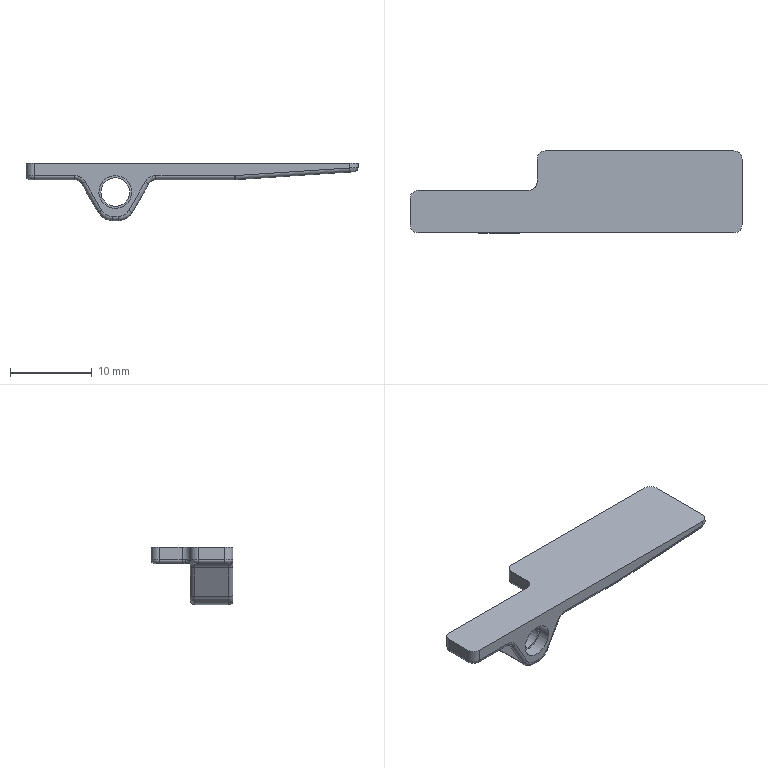NC program | Mastercam | posted with a generic post | part box 40.5 x 10 x 7 mm
Lines 1 to 1263 of 12178:
%
:0001()
(MATERIAL - ALUMINUM MM - 2024)
(T10|10 FEM |H10)
(T2|2 FEM |H2)
(T20|63 FEM |H20)
(T7|4 CHM |H7)
(T3|3 FEM |H3)
(T6|6 FEM |H6)
(T1|2 BM/BNOS |H1)
N100 G21
N102 G0 G17 G40 G80 G90 G94 G98
N104 G0 G28 G91 Z0.
N106 G0 G28 X0. Y0.
(10 FEM |TOOL - 10|DIA. OFF. - 10|LEN. - 10|TOOL DIA. - 10.)
N108 T10 M6
N110 G0 G54 G90 X20.25 Y-12. C0. B0. S6500 M3
N112 G43 H10 Z50.
N114 Z1.
N116 G1 Z-7. F600.
N118 Y-11. F1000.
N120 G3 X19.25 Y-10. I-1.
N122 G1 X-19.25
N124 G2 X-25.25 Y-4. J6.
N126 G1 Y-.8
N128 G2 X-19.25 Y5.2 I6.
N130 G1 X-9.629
N132 G2 X-3.75 Y10. I5.879 J-1.2
N134 G1 X19.25
N136 G2 X25.25 Y4. J-6.
N138 G1 Y-4.
N140 G2 X19.25 Y-10. I-6.
N142 G1 X18.75
N144 G3 X17.75 Y-11. J-1.
N146 G1 Y-12.
N148 G0 Z50.
N150 M5
N152 G0 G28 G91 Z0.
N154 G28
N156 M01
N158 G0 G17 G40 G80 G90 G94 G98
N160 G0 G28 G91 Z0.
(2 FEM |TOOL - 2|DIA. OFF. - 2|LEN. - 2|TOOL DIA. - 2.)
N162 T2 M6
N164 G0 G54 G90 X-10.121 Y1.6 C0. B0. S5000 M3
N166 G43 H2 Z50.
N168 Z1.
N170 G1 Z-7. F600.
N172 Y1.4
N174 G3 X-9.921 Y1.2 I.2
N176 G1 X-5.75
N178 Y4.
N180 G2 X-5.507 Y4.955 I2.
N182 G3 X-5.483 Y5.05 I-.176 J.095
N184 X-5.588 Y5.226 I-.2
N186 G1 X-5.764 Y5.321
N188 G0 Z50.
N190 M5
N192 G0 G28 G91 Z0.
N194 G28
N196 M01
N198 G0 G17 G40 G80 G90 G94 G98
N200 G0 G28 G91 Z0.
(63 FEM |TOOL - 20|DIA. OFF. - 20|LEN. - 20|TOOL DIA. - 63.)
N202 T20 M6
N204 G0 G54 G90 X0. Y-65.2 C0. B0. S4000 M3
N206 G43 H20 Z55.
N208 Z7.
N210 G1 Z4.623 F600.
N212 Y65.2 F2000.
N214 G0 Z54.623
N216 Y-65.2
N218 Z6.623
N220 G1 Z4.246 F600.
N222 Y65.2 F2000.
N224 G0 Z54.246
N226 Y-65.2
N228 Z6.246
N230 G1 Z3.869 F600.
N232 Y65.2 F2000.
N234 G0 Z53.869
N236 Y-65.2
N238 Z5.869
N240 G1 Z3.492 F600.
N242 Y65.2 F2000.
N244 G0 Z53.492
N246 Y-65.2
N248 Z5.492
N250 G1 Z3.115 F600.
N252 Y65.2 F2000.
N254 G0 Z53.115
N256 Y-65.2
N258 Z5.115
N260 G1 Z2.738 F600.
N262 Y65.2 F2000.
N264 G0 Z52.738
N266 Y-65.2
N268 Z4.738
N270 G1 Z2.362 F600.
N272 Y65.2 F2000.
N274 G0 Z52.362
N276 Y-65.2
N278 Z4.362
N280 G1 Z1.985 F600.
N282 Y65.2 F2000.
N284 G0 Z51.985
N286 Y-65.2
N288 Z3.985
N290 G1 Z1.608 F600.
N292 Y65.2 F2000.
N294 G0 Z51.608
N296 Y-65.2
N298 Z3.608
N300 G1 Z1.231 F600.
N302 Y65.2 F2000.
N304 G0 Z51.231
N306 Y-65.2
N308 Z3.231
N310 G1 Z.854 F600.
N312 Y65.2 F2000.
N314 G0 Z50.854
N316 Y-65.2
N318 Z2.854
N320 G1 Z.477 F600.
N322 Y65.2 F2000.
N324 G0 Z50.477
N326 Y-65.2
N328 Z2.477
N330 G1 Z.1 F600.
N332 Y65.2 F2000.
N334 G0 Z50.1
N336 Y-65.2
N338 Z2.1
N340 G1 Z0. F600.
N342 Y65.2 F1000.
N344 G0 Z50.
N346 M5
N348 G0 G28 G91 Z0.
N350 G28
N352 M01
N354 G0 G17 G40 G80 G90 G94 G98
N356 G0 G28 G91 Z0.
(4 CHM |TOOL - 7|DIA. OFF. - 7|LEN. - 7|TOOL DIA. - 4.)
N358 T7 M6
N360 G0 G54 G90 X19.65 Y-6.45 C0. B0. S6500 M3
N362 G43 H7 Z50.
N364 Z1.
N366 G1 Z-.7 F600.
N368 Y-6.05 F1000.
N370 G3 X19.25 Y-5.65 I-.4
N372 G1 X-3.75
N374 G2 X-5.4 Y-4. J1.65
N376 G1 Y-1.2
N378 G3 X-5.75 Y-.85 I-.35
N380 G1 X-19.25
N382 G2 X-20.9 Y.8 J1.65
N384 G1 Y4.
N386 G2 X-19.25 Y5.65 I1.65
N388 G1 X19.25
N390 G2 X20.9 Y4. J-1.65
N392 G1 Y-4.
N394 G2 X19.25 Y-5.65 I-1.65
N396 G3 X18.85 Y-6.05 J-.4
N398 G1 Y-6.45
N400 G0 Z50.
N402 M5
N404 G0 G28 G91 Z0.
N406 G28
N408 M01
N410 G0 G17 G40 G80 G90 G94 G98
N412 G0 G28 G91 Z0.
(3 FEM |TOOL - 3|DIA. OFF. - 3|LEN. - 3|TOOL DIA. - 3.)
N414 T3 M6
N416 G0 G54 G90 X-9.097 Y-.334 C0. B0. S6000 M3
N418 G43 H3 Z50.
N420 Z2.5
N422 G1 Z2. F600.
N424 X-9.091 Y-.33 Z1.839 F1000.
N426 X-9.075 Y-.321 Z1.68
N428 X-9.05 Y-.287 Z1.487
N430 X-9.015 Y-.239 Z1.299
N432 X-8.969 Y-.176 Z1.118
N434 X-8.952 Y-.094 Z.966
N436 X-8.932 Y0. Z.821
N438 X-8.95 Y.084 Z.711
N440 X-8.969 Y.176 Z.607
N442 X-9.021 Y.246 Z.523
N444 X-9.075 Y.321 Z.444
N446 X-9.148 Y.374 Z.375
N448 X-9.231 Y.401 Z.316
N450 X-9.318 Y.429 Z.261
N452 X-9.408 Z.212
N454 X-9.579 Y.374 Z.133
N456 X-9.712 Y.254 Z.074
N458 X-9.785 Y.089 Z.032
N460 Y-.089 Z.008
N462 X-9.712 Y-.254 Z0.
N464 X-9.579 Y-.374
N466 X-9.368 Y-.438
N468 X-9.23 Y-.41
N470 X-9.075 Y-.321
N472 X-8.969 Y-.176
N474 X-8.932 Y0.
N476 X-8.969 Y.176
N478 X-9.075 Y.321
N480 X-9.148 Y.374
N482 X-9.318 Y.429
N484 X-9.408
N486 X-9.579 Y.374
N488 X-9.712 Y.254
N490 X-9.785 Y.089
N492 Y-.089
N494 X-9.712 Y-.254
N496 X-9.587 Y-.366 Z-.016
N498 X-9.549 Y-.383 Z-.019
N500 X-9.388 Y-.432 Z-.035
N502 X-9.347 Y-.433 Z-.039
N504 X-9.265 Y-.417 Z-.047
N506 X-9.224 Y-.407 Z-.051
N508 X-9.078 Y-.323 Z-.066
N510 X-9.052 Y-.29 Z-.07
N512 X-8.978 Y-.188 Z-.082
N514 X-8.964 Y-.149 Z-.086
N516 X-8.937 Y-.026 Z-.098
N518 X-8.935 Y.015 Z-.101
N520 X-8.962 Y.139 Z-.113
N522 X-8.972 Y.179 Z-.117
N524 X-9.071 Y.316 Z-.133
N526 X-9.104 Y.342 Z-.137
N528 X-9.138 Y.366 Z-.141
N530 X-9.176 Y.383 Z-.144
N532 X-9.296 Y.422 Z-.156
N534 X-9.337 Y.429 Z-.16
N536 X-9.379 Z-.164
N538 X-9.421 Y.425 Z-.168
N540 X-9.541 Y.386 Z-.18
N542 X-9.58 Y.372 Z-.184
N544 X-9.705 Y.26 Z-.199
N546 X-9.726 Y.223 Z-.203
N548 X-9.777 Y.108 Z-.215
N550 X-9.785 Y.068 Z-.219
N552 Y-.059 Z-.23
N554 X-9.781 Y-.1 Z-.234
N556 X-9.712 Y-.254 Z-.25
N558 X-9.587 Y-.366 Z-.266
N560 X-9.549 Y-.383 Z-.269
N562 X-9.388 Y-.432 Z-.285
N564 X-9.347 Y-.433 Z-.289
N566 X-9.265 Y-.417 Z-.297
N568 X-9.224 Y-.407 Z-.301
N570 X-9.078 Y-.323 Z-.316
N572 X-9.052 Y-.29 Z-.32
N574 X-8.978 Y-.188 Z-.332
N576 X-8.964 Y-.149 Z-.336
N578 X-8.937 Y-.026 Z-.348
N580 X-8.935 Y.015 Z-.351
N582 X-8.962 Y.139 Z-.363
N584 X-8.972 Y.179 Z-.367
N586 X-9.071 Y.316 Z-.383
N588 X-9.104 Y.342 Z-.387
N590 X-9.138 Y.366 Z-.391
N592 X-9.176 Y.383 Z-.394
N594 X-9.296 Y.422 Z-.406
N596 X-9.337 Y.429 Z-.41
N598 X-9.379 Z-.414
N600 X-9.421 Y.425 Z-.418
N602 X-9.541 Y.386 Z-.43
N604 X-9.58 Y.372 Z-.434
N606 X-9.705 Y.26 Z-.449
N608 X-9.726 Y.223 Z-.453
N610 X-9.777 Y.108 Z-.465
N612 X-9.785 Y.068 Z-.469
N614 Y-.059 Z-.48
N616 X-9.781 Y-.1 Z-.484
N618 X-9.712 Y-.254 Z-.5
N620 X-9.587 Y-.366 Z-.516
N622 X-9.549 Y-.383 Z-.519
N624 X-9.388 Y-.432 Z-.535
N626 X-9.347 Y-.433 Z-.539
N628 X-9.265 Y-.417 Z-.547
N630 X-9.224 Y-.407 Z-.551
N632 X-9.078 Y-.323 Z-.566
N634 X-9.052 Y-.29 Z-.57
N636 X-8.978 Y-.188 Z-.582
N638 X-8.964 Y-.149 Z-.586
N640 X-8.937 Y-.026 Z-.598
N642 X-8.935 Y.015 Z-.601
N644 X-8.962 Y.139 Z-.613
N646 X-8.972 Y.179 Z-.617
N648 X-9.071 Y.316 Z-.633
N650 X-9.104 Y.342 Z-.637
N652 X-9.138 Y.366 Z-.641
N654 X-9.176 Y.383 Z-.644
N656 X-9.296 Y.422 Z-.656
N658 X-9.337 Y.429 Z-.66
N660 X-9.379 Z-.664
N662 X-9.421 Y.425 Z-.668
N664 X-9.541 Y.386 Z-.68
N666 X-9.58 Y.372 Z-.684
N668 X-9.705 Y.26 Z-.699
N670 X-9.726 Y.223 Z-.703
N672 X-9.777 Y.108 Z-.715
N674 X-9.785 Y.068 Z-.719
N676 Y-.059 Z-.73
N678 X-9.781 Y-.1 Z-.734
N680 X-9.712 Y-.254 Z-.75
N682 X-9.587 Y-.366 Z-.766
N684 X-9.549 Y-.383 Z-.769
N686 X-9.388 Y-.432 Z-.785
N688 X-9.347 Y-.433 Z-.789
N690 X-9.265 Y-.417 Z-.797
N692 X-9.224 Y-.407 Z-.801
N694 X-9.078 Y-.323 Z-.816
N696 X-9.052 Y-.29 Z-.82
N698 X-8.978 Y-.188 Z-.832
N700 X-8.964 Y-.149 Z-.836
N702 X-8.937 Y-.026 Z-.848
N704 X-8.935 Y.015 Z-.851
N706 X-8.962 Y.139 Z-.863
N708 X-8.972 Y.179 Z-.867
N710 X-9.071 Y.316 Z-.883
N712 X-9.104 Y.342 Z-.887
N714 X-9.138 Y.366 Z-.891
N716 X-9.176 Y.383 Z-.894
N718 X-9.296 Y.422 Z-.906
N720 X-9.337 Y.429 Z-.91
N722 X-9.379 Z-.914
N724 X-9.421 Y.425 Z-.918
N726 X-9.541 Y.386 Z-.93
N728 X-9.58 Y.372 Z-.934
N730 X-9.705 Y.26 Z-.949
N732 X-9.726 Y.223 Z-.953
N734 X-9.777 Y.108 Z-.965
N736 X-9.785 Y.068 Z-.969
N738 Y-.059 Z-.98
N740 X-9.781 Y-.1 Z-.984
N742 X-9.712 Y-.254 Z-1.
N744 X-9.587 Y-.366 Z-1.016
N746 X-9.549 Y-.383 Z-1.019
N748 X-9.388 Y-.432 Z-1.035
N750 X-9.347 Y-.433 Z-1.039
N752 X-9.265 Y-.417 Z-1.047
N754 X-9.224 Y-.407 Z-1.051
N756 X-9.078 Y-.323 Z-1.066
N758 X-9.052 Y-.29 Z-1.07
N760 X-8.978 Y-.188 Z-1.082
N762 X-8.964 Y-.149 Z-1.086
N764 X-8.937 Y-.026 Z-1.098
N766 X-8.935 Y.015 Z-1.101
N768 X-8.962 Y.139 Z-1.113
N770 X-8.972 Y.179 Z-1.117
N772 X-9.071 Y.316 Z-1.133
N774 X-9.104 Y.342 Z-1.137
N776 X-9.138 Y.366 Z-1.141
N778 X-9.176 Y.383 Z-1.144
N780 X-9.296 Y.422 Z-1.156
N782 X-9.337 Y.429 Z-1.16
N784 X-9.379 Z-1.164
N786 X-9.421 Y.425 Z-1.168
N788 X-9.541 Y.386 Z-1.18
N790 X-9.58 Y.372 Z-1.184
N792 X-9.705 Y.26 Z-1.199
N794 X-9.726 Y.223 Z-1.203
N796 X-9.777 Y.108 Z-1.215
N798 X-9.785 Y.068 Z-1.219
N800 Y-.059 Z-1.23
N802 X-9.781 Y-.1 Z-1.234
N804 X-9.712 Y-.254 Z-1.25
N806 X-9.578 Y-.353 Z-1.266
N808 X-9.54 Y-.366 Z-1.27
N810 X-9.502 Y-.374 Z-1.273
N812 X-9.421 Y-.39 Z-1.281
N814 X-9.386 Y-.397 Z-1.285
N816 X-9.351 Y-.394 Z-1.288
N818 X-9.237 Y-.357 Z-1.301
N820 X-9.122 Y-.271 Z-1.316
N822 X-9.099 Y-.239 Z-1.32
N824 X-9.053 Y-.153 Z-1.331
N826 X-9.041 Y-.113 Z-1.336
N828 X-9.035 Y-.026 Z-1.347
N830 X-9.037 Y.015 Z-1.352
N832 X-9.055 Y.072 Z-1.359
N834 X-9.08 Y.129 Z-1.367
N836 X-9.121 Y.179 Z-1.375
N838 X-9.158 Y.213 Z-1.381
N840 X-9.193 Y.237 Z-1.387
N842 X-9.217 Y.25 Z-1.391
N844 X-9.322 Y.264 Z-1.405
N846 X-9.387 Y.265 Z-1.414
N848 X-9.476 Y.22 Z-1.43
N850 X-9.501 Y.198 Z-1.435
N852 X-9.534 Y.155 Z-1.445
N854 X-9.555 Y.116 Z-1.452
N856 X-9.551 Y.077 Z-1.459
N858 X-9.557 Y.022 Z-1.469
N860 X-9.552 Y.01 Z-1.471
N862 X-9.547 Y-.032 Z-1.479
N864 X-9.539 Y-.06 Z-1.484
N866 X-9.537 Z-1.485
N868 X-9.532 Y-.071 Z-1.487
N870 X-9.528 Y-.078 Z-1.489
N872 X-9.52 Y-.089 Z-1.492
N874 X-9.496 Y-.123 Z-1.5
N876 X-9.438 Y-.163 Z-1.516
N878 X-9.405 Y-.175 Z-1.523
N880 X-9.371 Y-.183 Z-1.531
N882 X-9.303 Y-.166 Z-1.547
N884 X-9.271 Y-.153 Z-1.555
N886 X-9.218 Y-.107 Z-1.57
N888 X-9.189 Y-.043 Z-1.586
N890 X-9.187 Y.027 Z-1.602
N892 X-9.197 Y.06 Z-1.609
N894 X-9.212 Y.092 Z-1.617
N896 X-9.232 Y.12 Z-1.625
N898 X-9.259 Y.143 Z-1.633
N900 X-9.287 Y.161 Z-1.64
N902 X-9.357 Y.173 Z-1.656
N904 X-9.392 Y.178 Z-1.664
N906 X-9.457 Y.153 Z-1.68
N908 X-9.483 Y.13 Z-1.688
N910 X-9.508 Y.104 Z-1.695
N912 X-9.524 Y.074 Z-1.703
N914 X-9.536 Y.041 Z-1.711
N916 X-9.542 Y.007 Z-1.719
N918 X-9.532 Y-.062 Z-1.734
N920 X-9.496 Y-.123 Z-1.75
N922 X-9.438 Y-.163 Z-1.766
N924 X-9.405 Y-.175 Z-1.773
N926 X-9.371 Y-.183 Z-1.781
N928 X-9.303 Y-.166 Z-1.797
N930 X-9.271 Y-.153 Z-1.805
N932 X-9.218 Y-.107 Z-1.82
N934 X-9.189 Y-.043 Z-1.836
N936 X-9.187 Y.027 Z-1.852
N938 X-9.197 Y.06 Z-1.859
N940 X-9.212 Y.092 Z-1.867
N942 X-9.232 Y.12 Z-1.875
N944 X-9.259 Y.143 Z-1.883
N946 X-9.287 Y.161 Z-1.89
N948 X-9.357 Y.173 Z-1.906
N950 X-9.392 Y.178 Z-1.914
N952 X-9.457 Y.153 Z-1.93
N954 X-9.483 Y.13 Z-1.938
N956 X-9.508 Y.104 Z-1.945
N958 X-9.524 Y.074 Z-1.953
N960 X-9.536 Y.041 Z-1.961
N962 X-9.542 Y.007 Z-1.969
N964 X-9.532 Y-.062 Z-1.984
N966 X-9.496 Y-.123 Z-2.
N968 X-9.438 Y-.163 Z-2.016
N970 X-9.405 Y-.175 Z-2.023
N972 X-9.371 Y-.183 Z-2.031
N974 X-9.303 Y-.166 Z-2.047
N976 X-9.271 Y-.153 Z-2.055
N978 X-9.218 Y-.107 Z-2.07
N980 X-9.189 Y-.043 Z-2.086
N982 X-9.187 Y.027 Z-2.102
N984 X-9.197 Y.06 Z-2.109
N986 X-9.212 Y.092 Z-2.117
N988 X-9.232 Y.12 Z-2.125
N990 X-9.259 Y.143 Z-2.133
N992 X-9.287 Y.161 Z-2.14
N994 X-9.357 Y.173 Z-2.156
N996 X-9.392 Y.178 Z-2.164
N998 X-9.457 Y.153 Z-2.18
N1000 X-9.483 Y.13 Z-2.188
N1002 X-9.508 Y.104 Z-2.195
N1004 X-9.524 Y.074 Z-2.203
N1006 X-9.536 Y.041 Z-2.211
N1008 X-9.542 Y.007 Z-2.219
N1010 X-9.532 Y-.062 Z-2.234
N1012 X-9.496 Y-.123 Z-2.25
N1014 X-9.438 Y-.163 Z-2.266
N1016 X-9.405 Y-.175 Z-2.273
N1018 X-9.371 Y-.183 Z-2.281
N1020 X-9.303 Y-.166 Z-2.297
N1022 X-9.271 Y-.153 Z-2.305
N1024 X-9.218 Y-.107 Z-2.32
N1026 X-9.189 Y-.043 Z-2.336
N1028 X-9.187 Y.027 Z-2.352
N1030 X-9.197 Y.06 Z-2.359
N1032 X-9.212 Y.092 Z-2.367
N1034 X-9.232 Y.12 Z-2.375
N1036 X-9.259 Y.143 Z-2.383
N1038 X-9.287 Y.161 Z-2.39
N1040 X-9.357 Y.173 Z-2.406
N1042 X-9.392 Y.178 Z-2.414
N1044 X-9.457 Y.153 Z-2.43
N1046 X-9.483 Y.13 Z-2.438
N1048 X-9.508 Y.104 Z-2.445
N1050 X-9.524 Y.074 Z-2.453
N1052 X-9.536 Y.041 Z-2.461
N1054 X-9.542 Y.007 Z-2.469
N1056 X-9.532 Y-.062 Z-2.484
N1058 X-9.496 Y-.123 Z-2.5
N1060 X-9.438 Y-.163 Z-2.516
N1062 X-9.405 Y-.175 Z-2.523
N1064 X-9.371 Y-.183 Z-2.531
N1066 X-9.303 Y-.166 Z-2.547
N1068 X-9.271 Y-.153 Z-2.555
N1070 X-9.218 Y-.107 Z-2.57
N1072 X-9.189 Y-.043 Z-2.586
N1074 X-9.187 Y.027 Z-2.602
N1076 X-9.197 Y.06 Z-2.609
N1078 X-9.212 Y.092 Z-2.617
N1080 X-9.232 Y.12 Z-2.625
N1082 X-9.259 Y.143 Z-2.633
N1084 X-9.287 Y.161 Z-2.64
N1086 X-9.357 Y.173 Z-2.656
N1088 X-9.392 Y.178 Z-2.664
N1090 X-9.457 Y.153 Z-2.68
N1092 X-9.483 Y.13 Z-2.688
N1094 X-9.508 Y.104 Z-2.695
N1096 X-9.524 Y.074 Z-2.703
N1098 X-9.536 Y.041 Z-2.711
N1100 X-9.542 Y.007 Z-2.719
N1102 X-9.532 Y-.062 Z-2.734
N1104 X-9.496 Y-.123 Z-2.75
N1106 X-9.438 Y-.163 Z-2.766
N1108 X-9.405 Y-.175 Z-2.773
N1110 X-9.371 Y-.183 Z-2.781
N1112 X-9.303 Y-.166 Z-2.797
N1114 X-9.271 Y-.153 Z-2.805
N1116 X-9.218 Y-.107 Z-2.82
N1118 X-9.189 Y-.043 Z-2.836
N1120 X-9.187 Y.027 Z-2.852
N1122 X-9.197 Y.06 Z-2.859
N1124 X-9.212 Y.092 Z-2.867
N1126 X-9.232 Y.12 Z-2.875
N1128 X-9.259 Y.143 Z-2.883
N1130 X-9.287 Y.161 Z-2.89
N1132 X-9.357 Y.173 Z-2.906
N1134 X-9.392 Y.178 Z-2.914
N1136 X-9.457 Y.153 Z-2.93
N1138 X-9.483 Y.13 Z-2.938
N1140 X-9.508 Y.104 Z-2.945
N1142 X-9.524 Y.074 Z-2.953
N1144 X-9.536 Y.041 Z-2.961
N1146 X-9.542 Y.007 Z-2.969
N1148 X-9.532 Y-.062 Z-2.984
N1150 X-9.496 Y-.123 Z-3.
N1152 X-9.438 Y-.163 Z-3.016
N1154 X-9.405 Y-.175 Z-3.023
N1156 X-9.371 Y-.183 Z-3.031
N1158 X-9.303 Y-.166 Z-3.047
N1160 X-9.271 Y-.153 Z-3.055
N1162 X-9.218 Y-.107 Z-3.07
N1164 X-9.189 Y-.043 Z-3.086
N1166 X-9.187 Y.027 Z-3.102
N1168 X-9.197 Y.06 Z-3.109
N1170 X-9.212 Y.092 Z-3.117
N1172 X-9.232 Y.12 Z-3.125
N1174 X-9.259 Y.143 Z-3.133
N1176 X-9.287 Y.161 Z-3.14
N1178 X-9.357 Y.173 Z-3.156
N1180 X-9.392 Y.178 Z-3.164
N1182 X-9.457 Y.153 Z-3.18
N1184 X-9.483 Y.13 Z-3.188
N1186 X-9.508 Y.104 Z-3.195
N1188 X-9.524 Y.074 Z-3.203
N1190 X-9.536 Y.041 Z-3.211
N1192 X-9.542 Y.007 Z-3.219
N1194 X-9.532 Y-.062 Z-3.234
N1196 X-9.496 Y-.123 Z-3.25
N1198 X-9.438 Y-.163 Z-3.266
N1200 X-9.405 Y-.175 Z-3.273
N1202 X-9.371 Y-.183 Z-3.281
N1204 X-9.303 Y-.166 Z-3.297
N1206 X-9.271 Y-.153 Z-3.305
N1208 X-9.218 Y-.107 Z-3.32
N1210 X-9.189 Y-.043 Z-3.336
N1212 X-9.187 Y.027 Z-3.352
N1214 X-9.197 Y.06 Z-3.359
N1216 X-9.212 Y.092 Z-3.367
N1218 X-9.232 Y.12 Z-3.375
N1220 X-9.259 Y.143 Z-3.383
N1222 X-9.287 Y.161 Z-3.39
N1224 X-9.357 Y.173 Z-3.406
N1226 X-9.392 Y.178 Z-3.414
N1228 X-9.457 Y.153 Z-3.43
N1230 X-9.483 Y.13 Z-3.438
N1232 X-9.508 Y.104 Z-3.445
N1234 X-9.524 Y.074 Z-3.453
N1236 X-9.536 Y.041 Z-3.461
N1238 X-9.542 Y.007 Z-3.469
N1240 X-9.532 Y-.062 Z-3.484
N1242 X-9.496 Y-.123 Z-3.5
N1244 X-9.438 Y-.163 Z-3.516
N1246 X-9.405 Y-.175 Z-3.523
N1248 X-9.371 Y-.183 Z-3.531
N1250 X-9.303 Y-.166 Z-3.547
N1252 X-9.271 Y-.153 Z-3.555
N1254 X-9.218 Y-.107 Z-3.57
N1256 X-9.189 Y-.043 Z-3.586
N1258 X-9.187 Y.027 Z-3.602
N1260 X-9.197 Y.06 Z-3.609
N1262 X-9.212 Y.092 Z-3.617
N1264 X-9.232 Y.12 Z-3.625
N1266 X-9.259 Y.143 Z-3.633
N1268 X-9.287 Y.161 Z-3.64
N1270 X-9.357 Y.173 Z-3.656
N1272 X-9.392 Y.178 Z-3.664
N1274 X-9.457 Y.153 Z-3.68
N1276 X-9.483 Y.13 Z-3.688
N1278 X-9.508 Y.104 Z-3.695
N1280 X-9.524 Y.074 Z-3.703
N1282 X-9.536 Y.041 Z-3.711
N1284 X-9.542 Y.007 Z-3.719
N1286 X-9.532 Y-.062 Z-3.734
N1288 X-9.496 Y-.123 Z-3.75
N1290 X-9.438 Y-.163 Z-3.766
N1292 X-9.405 Y-.175 Z-3.773
N1294 X-9.371 Y-.183 Z-3.781
N1296 X-9.303 Y-.166 Z-3.797
N1298 X-9.271 Y-.153 Z-3.805
N1300 X-9.218 Y-.107 Z-3.82
N1302 X-9.189 Y-.043 Z-3.836
N1304 X-9.187 Y.027 Z-3.852
N1306 X-9.197 Y.06 Z-3.859
N1308 X-9.212 Y.092 Z-3.867
N1310 X-9.232 Y.12 Z-3.875
N1312 X-9.259 Y.143 Z-3.883
N1314 X-9.287 Y.161 Z-3.89
N1316 X-9.357 Y.173 Z-3.906
N1318 X-9.392 Y.178 Z-3.914
N1320 X-9.457 Y.153 Z-3.93
N1322 X-9.483 Y.13 Z-3.938
N1324 X-9.508 Y.104 Z-3.945
N1326 X-9.524 Y.074 Z-3.953
N1328 X-9.536 Y.041 Z-3.961
N1330 X-9.542 Y.007 Z-3.969
N1332 X-9.532 Y-.062 Z-3.984
N1334 X-9.496 Y-.123 Z-4.
N1336 X-9.438 Y-.163 Z-4.016
N1338 X-9.405 Y-.175 Z-4.023
N1340 X-9.371 Y-.183 Z-4.031
N1342 X-9.303 Y-.166 Z-4.047
N1344 X-9.271 Y-.153 Z-4.055
N1346 X-9.218 Y-.107 Z-4.07
N1348 X-9.189 Y-.043 Z-4.086
N1350 X-9.187 Y.027 Z-4.102
N1352 X-9.197 Y.06 Z-4.109
N1354 X-9.212 Y.092 Z-4.117
N1356 X-9.232 Y.12 Z-4.125
N1358 X-9.259 Y.143 Z-4.133
N1360 X-9.287 Y.161 Z-4.14
N1362 X-9.357 Y.173 Z-4.156
N1364 X-9.392 Y.178 Z-4.164
N1366 X-9.457 Y.153 Z-4.18
N1368 X-9.483 Y.13 Z-4.188
N1370 X-9.508 Y.104 Z-4.195
N1372 X-9.524 Y.074 Z-4.203
N1374 X-9.536 Y.041 Z-4.211
N1376 X-9.542 Y.007 Z-4.219
N1378 X-9.532 Y-.062 Z-4.234
N1380 X-9.496 Y-.123 Z-4.25
N1382 X-9.438 Y-.163 Z-4.266
N1384 X-9.405 Y-.175 Z-4.273
N1386 X-9.371 Y-.183 Z-4.281
N1388 X-9.303 Y-.166 Z-4.297
N1390 X-9.271 Y-.153 Z-4.305
N1392 X-9.218 Y-.107 Z-4.32
N1394 X-9.189 Y-.043 Z-4.336
N1396 X-9.187 Y.027 Z-4.352
N1398 X-9.197 Y.06 Z-4.359
N1400 X-9.212 Y.092 Z-4.367
N1402 X-9.232 Y.12 Z-4.375
N1404 X-9.259 Y.143 Z-4.383
N1406 X-9.287 Y.161 Z-4.39
N1408 X-9.357 Y.173 Z-4.406
N1410 X-9.392 Y.178 Z-4.414
N1412 X-9.457 Y.153 Z-4.43
N1414 X-9.483 Y.13 Z-4.438
N1416 X-9.508 Y.104 Z-4.445
N1418 X-9.524 Y.074 Z-4.453
N1420 X-9.536 Y.041 Z-4.461
N1422 X-9.542 Y.007 Z-4.469
N1424 X-9.532 Y-.062 Z-4.484
N1426 X-9.496 Y-.123 Z-4.5
N1428 X-9.438 Y-.163 Z-4.516
N1430 X-9.405 Y-.175 Z-4.523
N1432 X-9.371 Y-.183 Z-4.531
N1434 X-9.303 Y-.166 Z-4.547
N1436 X-9.271 Y-.153 Z-4.555
N1438 X-9.218 Y-.107 Z-4.57
N1440 X-9.189 Y-.043 Z-4.586
N1442 X-9.187 Y.027 Z-4.602
N1444 X-9.197 Y.06 Z-4.609
N1446 X-9.212 Y.092 Z-4.617
N1448 X-9.232 Y.12 Z-4.625
N1450 X-9.259 Y.143 Z-4.633
N1452 X-9.287 Y.161 Z-4.64
N1454 X-9.357 Y.173 Z-4.656
N1456 X-9.392 Y.178 Z-4.664
N1458 X-9.457 Y.153 Z-4.68
N1460 X-9.483 Y.13 Z-4.688
N1462 X-9.508 Y.104 Z-4.695
N1464 X-9.524 Y.074 Z-4.703
N1466 X-9.536 Y.041 Z-4.711
N1468 X-9.542 Y.007 Z-4.719
N1470 X-9.532 Y-.062 Z-4.734
N1472 X-9.496 Y-.123 Z-4.75
N1474 X-9.438 Y-.163 Z-4.766
N1476 X-9.405 Y-.175 Z-4.773
N1478 X-9.371 Y-.183 Z-4.781
N1480 X-9.303 Y-.166 Z-4.797
N1482 X-9.271 Y-.153 Z-4.805
N1484 X-9.218 Y-.107 Z-4.82
N1486 X-9.189 Y-.043 Z-4.836
N1488 X-9.187 Y.027 Z-4.852
N1490 X-9.197 Y.06 Z-4.859
N1492 X-9.212 Y.092 Z-4.867
N1494 X-9.232 Y.12 Z-4.875
N1496 X-9.259 Y.143 Z-4.883
N1498 X-9.287 Y.161 Z-4.89
N1500 X-9.357 Y.173 Z-4.906
N1502 X-9.392 Y.178 Z-4.914
N1504 X-9.457 Y.153 Z-4.93
N1506 X-9.483 Y.13 Z-4.938
N1508 X-9.508 Y.104 Z-4.945
N1510 X-9.524 Y.074 Z-4.953
N1512 X-9.536 Y.041 Z-4.961
N1514 X-9.542 Y.007 Z-4.969
N1516 X-9.532 Y-.062 Z-4.984
N1518 X-9.496 Y-.123 Z-5.
N1520 X-9.438 Y-.163 Z-5.016
N1522 X-9.405 Y-.175 Z-5.023
N1524 X-9.371 Y-.183 Z-5.031
N1526 X-9.303 Y-.166 Z-5.047
N1528 X-9.271 Y-.153 Z-5.055
N1530 X-9.218 Y-.107 Z-5.07
N1532 X-9.189 Y-.043 Z-5.086
N1534 X-9.187 Y.027 Z-5.102
N1536 X-9.197 Y.06 Z-5.109
N1538 X-9.212 Y.092 Z-5.117
N1540 X-9.232 Y.12 Z-5.125
N1542 X-9.259 Y.143 Z-5.133
N1544 X-9.287 Y.161 Z-5.14
N1546 X-9.357 Y.173 Z-5.156
N1548 X-9.392 Y.178 Z-5.164
N1550 X-9.457 Y.153 Z-5.18
N1552 X-9.483 Y.13 Z-5.188
N1554 X-9.508 Y.104 Z-5.195
N1556 X-9.524 Y.074 Z-5.203
N1558 X-9.536 Y.041 Z-5.211
N1560 X-9.542 Y.007 Z-5.219
N1562 X-9.532 Y-.062 Z-5.234
N1564 X-9.496 Y-.123 Z-5.25
N1566 X-9.438 Y-.163 Z-5.266
N1568 X-9.405 Y-.175 Z-5.273
N1570 X-9.371 Y-.183 Z-5.281
N1572 X-9.303 Y-.166 Z-5.297
N1574 X-9.271 Y-.153 Z-5.305
N1576 X-9.218 Y-.107 Z-5.32
N1578 X-9.189 Y-.043 Z-5.336
N1580 X-9.187 Y.027 Z-5.352
N1582 X-9.197 Y.06 Z-5.359
N1584 X-9.212 Y.092 Z-5.367
N1586 X-9.232 Y.12 Z-5.375
N1588 X-9.259 Y.143 Z-5.383
N1590 X-9.287 Y.161 Z-5.39
N1592 X-9.357 Y.173 Z-5.406
N1594 X-9.392 Y.178 Z-5.414
N1596 X-9.457 Y.153 Z-5.43
N1598 X-9.483 Y.13 Z-5.438
N1600 X-9.508 Y.104 Z-5.445
N1602 X-9.524 Y.074 Z-5.453
N1604 X-9.536 Y.041 Z-5.461
N1606 X-9.542 Y.007 Z-5.469
N1608 X-9.532 Y-.062 Z-5.484
N1610 X-9.496 Y-.123 Z-5.5
N1612 X-9.495 Y-.124
N1614 X-9.431 Y-.168
N1616 X-9.373 Y-.184
N1618 X-9.279 Y-.16
N1620 X-9.22 Y-.11
N1622 X-9.187 Y-.039
N1624 Y.039
N1626 X-9.22 Y.11
N1628 X-9.279 Y.16
N1630 X-9.391 Y.179
N1632 X-9.465 Y.15
N1634 X-9.518 Y.093
N1636 X-9.543 Y.019
N1638 X-9.534 Y-.059
N1640 X-9.496 Y-.123
N1642 X-9.495 Y-.124
N1644 X-9.431 Y-.168 Z-5.498
N1646 X-9.373 Y-.184 Z-5.495
N1648 X-9.279 Y-.16 Z-5.486
N1650 X-9.22 Y-.11 Z-5.475
N1652 X-9.187 Y-.039 Z-5.461
N1654 Y.039 Z-5.444
N1656 X-9.22 Y.11 Z-5.423
N1658 X-9.279 Y.16 Z-5.4
N1660 X-9.391 Y.179 Z-5.359
N1662 X-9.465 Y.15 Z-5.325
N1664 X-9.518 Y.093 Z-5.288
N1666 X-9.543 Y.019 Z-5.247
N1668 X-9.534 Y-.059 Z-5.201
N1670 X-9.496 Y-.123 Z-5.152
N1672 X-9.495 Y-.124 Z-5.151
N1674 X-9.431 Y-.168 Z-5.096
N1676 X-9.373 Y-.184 Z-5.048
N1678 X-9.279 Y-.16 Z-4.963
N1680 X-9.22 Y-.11 Z-4.887
N1682 X-9.187 Y-.039 Z-4.801
N1684 Y.039 Z-4.704
N1686 X-9.22 Y.11 Z-4.593
N1688 X-9.279 Y.16 Z-4.465
N1690 X-9.339 Y.17 Z-4.344
N1692 X-9.391 Y.179 Z-4.22
N1694 X-9.432 Y.163 Z-4.094
N1696 X-9.465 Y.15 Z-3.966
N1698 X-9.486 Y.128 Z-3.812
N1700 X-9.498 Y.114 Z-3.656
N1702 X-9.502 Y.11 Z-3.5
N1704 Z-3. F1200.
N1706 G0 Z50.
N1708 X-9.663 Y.09
N1710 Z-.5
N1712 G1 Z-1.5 F600.
N1714 Y-.21 F500.
N1716 G3 X-9.363 Y-.51 I.3
N1718 X-8.853 Y0. J.51
N1720 X-9.363 Y.51 I-.51
N1722 X-9.873 Y0. J-.51
N1724 X-9.363 Y-.51 I.51
N1726 X-9.063 Y-.21 J.3
N1728 G1 Y.09
N1730 G0 Z50.
N1732 X-9.363 Y-.26
N1734 Z-.5
N1736 G1 Z-1.5 F600.
N1738 G3 X-9.103 Y0. Z-1.75 J.26 F500.
N1740 X-9.363 Y.26 Z-2. I-.26
N1742 X-9.623 Y0. Z-2.25 J-.26
N1744 X-9.363 Y-.26 Z-2.5 I.26
N1746 X-9.103 Y0. Z-2.75 J.26
N1748 X-9.363 Y.26 Z-3. I-.26
N1750 X-9.623 Y0. Z-3.25 J-.26
N1752 X-9.363 Y-.26 Z-3.5 I.26
N1754 X-9.103 Y0. Z-3.75 J.26
N1756 X-9.363 Y.26 Z-4. I-.26
N1758 X-9.623 Y0. Z-4.25 J-.26
N1760 X-9.363 Y-.26 Z-4.5 I.26
N1762 X-9.103 Y0. Z-4.75 J.26
N1764 X-9.363 Y.26 Z-5. I-.26
N1766 X-9.623 Y0. Z-5.25 J-.26
N1768 X-9.363 Y-.26 Z-5.5 I.26
N1770 X-9.103 Y0. J.26
N1772 X-9.363 Y.26 I-.26
N1774 X-9.623 Y0. J-.26
N1776 X-9.363 Y-.26 I.26
N1778 G0 Z50.
N1780 M5
N1782 G0 G28 G91 Z0.
N1784 G28
N1786 M01
N1788 G0 G17 G40 G80 G90 G94 G98
N1790 G0 G28 G91 Z0.
(4 CHM |TOOL - 7|DIA. OFF. - 7|LEN. - 7|TOOL DIA. - 4.)
N1792 T7 M6
N1794 G0 G54 G90 X-9.763 Y-.56 C0. B0. S6500 M3
N1796 G43 H7 Z50.
N1798 Z1.
N1800 G1 Z-.7 F600.
N1802 Y-.96 F1000.
N1804 G3 X-9.363 Y-1.36 I.4
N1806 X-8.003 Y0. J1.36
N1808 X-9.363 Y1.36 I-1.36
N1810 X-10.723 Y0. J-1.36
N1812 X-9.363 Y-1.36 I1.36
N1814 X-8.963 Y-.96 J.4
N1816 G1 Y-.56
N1818 G0 Z50.
N1820 M5
N1822 G0 G28 G91 Z0.
N1824 G28
N1826 M01
N1828 G0 G17 G40 G80 G90 G94 G98
N1830 G0 G28 G91 Z0.
(3 FEM |TOOL - 3|DIA. OFF. - 3|LEN. - 3|TOOL DIA. - 3.)
N1832 T3 M6
N1834 G0 G54 G90 X10.261 Y.804 C0. B0. S7000 M3
N1836 G43 H3 Z50.
N1838 Z1.
N1840 G1 Z.175 F600.
N1842 X8.611 Z.122 F3000.
N1844 X7.565 Z.089
N1846 X6.961 Z.069
N1848 X5.311 Z.017
N1850 X3.661 Z-.036
N1852 X2.011 Z-.089
N1854 X.361 Z-.142
N1856 X-1.342 Z-.194
N1858 G2 X-1.285 Y.695 I-6.467 J-3.447
N1860 X-.715 Y-.804 Z-.246 I-6.524 J-3.338
N1862 G1 X-.596 Z-.247
N1864 X1.054 Z-.3
N1866 X16.054
N1868 Y.804
N1870 X7.565
N1872 X-1.342
N1874 G2 X-.715 Y-.804 I-6.467 J-3.447
N1876 G1 X1.054
N1878 G2 X1.314 Y-1.004 J-.268
N1880 G1 X1.599 Y-2.094
N1882 G3 X1.859 Y-2.294 I.26 J.068
N1884 G1 X17.544
N1886 Y2.294
N1888 X7.565
N1890 X-5.366
N1892 G2 X-2.045 Y-2.294 I-1.626 J-4.672
N1894 G1 X1.859
N1896 G2 X2.11 Y-2.468 J-.268
N1898 G1 X2.412 Y-3.276
N1900 G3 X2.663 Y-3.45 I.251 J.094
N1902 G1 X17.702
N1904 G2 X17.892 Y-3.44 I.19 J-1.845
N1906 X19.1 Y-3.888 J-1.855
N1908 G1 X18.798 Y-3.27
N1910 X18.707 Y-2.885
N1912 X18.7 Y-1.346
N1914 X18.707 Y2.885
N1916 X18.798 Y3.27
N1918 X19.1 Y3.888
N1920 G2 X18.087 Y3.453 I-1.226 J1.46
N1922 G1 X17.702 Y3.45
N1924 X-12.288
N1926 X-18.087 Y3.453
N1928 G2 X-19.1 Y3.888 I.213 J1.895
N1930 G1 X-18.856 Y3.409
N1932 X-18.74 Y3.08
N1934 G2 X-18.699 Y2.244 I-8.568 J-.836
N1936 X-18.7 Y2.116 I-8.609
N1938 X-19.13 Y.962 I-1.794 J.011
N1940 G1 X-19.128 Y.907
N1942 X-19.108
N1944 G2 X-18.472 Y1.27 I2.712 J-4.017
N1946 G1 X-18.087 Y1.347
N1948 X-17.702 Y1.35
N1950 X-6.927
N1952 G2 X-6.832 Y1.351 I.095 J-3.858
N1954 X-5.003 Y.89 J-3.859
N1956 X-3.305 Y-1.346 I-1.84 J-3.159
N1958 X-3.198 Y-2.531 I-6.488 J-1.185
N1960 X-3.207 Y-2.885 I-6.595
N1962 X-3.627 Y-3.835 I-1.895 J.27
N1964 G1 X-3.463 Y-3.792
N1966 X-3.079 Y-3.571
N1968 X-2.694 Y-3.464
N1970 X-2.309 Y-3.45
N1972 X2.663
N1974 G0 Z50.
N1976 X10.261 Y.804
N1978 Z.7
N1980 G1 Z-.125 F600.
N1982 X8.611 Z-.178 F3000.
N1984 X7.565 Z-.211
N1986 X6.961 Z-.231
N1988 X5.311 Z-.283
N1990 X3.661 Z-.336
N1992 X2.011 Z-.389
N1994 X.361 Z-.442
N1996 X-1.342 Z-.494
N1998 G2 X-1.285 Y.695 I-6.467 J-3.447
N2000 X-.715 Y-.804 Z-.546 I-6.524 J-3.338
N2002 G1 X-.596 Z-.547
N2004 X1.054 Z-.6
N2006 X16.054
N2008 Y.804
N2010 X7.565
N2012 X-1.342
N2014 G2 X-.715 Y-.804 I-6.467 J-3.447
N2016 G1 X1.054
N2018 G2 X1.314 Y-1.004 J-.268
N2020 G1 X1.599 Y-2.094
N2022 G3 X1.859 Y-2.294 I.26 J.068
N2024 G1 X17.544
N2026 Y2.294
N2028 X7.565
N2030 X-5.366
N2032 G2 X-2.045 Y-2.294 I-1.626 J-4.672
N2034 G1 X1.859
N2036 G2 X2.11 Y-2.468 J-.268
N2038 G1 X2.412 Y-3.276
N2040 G3 X2.663 Y-3.45 I.251 J.094
N2042 G1 X17.702
N2044 G2 X17.892 Y-3.44 I.19 J-1.845
N2046 X19.1 Y-3.888 J-1.855
N2048 G1 X18.798 Y-3.27
N2050 X18.707 Y-2.885
N2052 X18.7 Y-1.346
N2054 X18.707 Y2.885
N2056 X18.798 Y3.27
N2058 X19.1 Y3.888
N2060 G2 X18.087 Y3.453 I-1.226 J1.46
N2062 G1 X17.702 Y3.45
N2064 X-12.288
N2066 X-18.087 Y3.453
N2068 G2 X-19.1 Y3.888 I.213 J1.895
N2070 G1 X-18.856 Y3.409
N2072 X-18.74 Y3.08
N2074 G2 X-18.699 Y2.244 I-8.568 J-.836
N2076 X-18.7 Y2.116 I-8.609
N2078 X-19.13 Y.962 I-1.794 J.011
N2080 G1 X-19.128 Y.907
N2082 X-19.108
N2084 G2 X-18.472 Y1.27 I2.712 J-4.017
N2086 G1 X-18.087 Y1.347
N2088 X-17.702 Y1.35
N2090 X-6.927
N2092 G2 X-6.832 Y1.351 I.095 J-3.858
N2094 X-5.003 Y.89 J-3.859
N2096 X-3.305 Y-1.346 I-1.84 J-3.159
N2098 X-3.198 Y-2.531 I-6.488 J-1.185
N2100 X-3.207 Y-2.885 I-6.595
N2102 X-3.627 Y-3.835 I-1.895 J.27
N2104 G1 X-3.463 Y-3.792
N2106 X-3.079 Y-3.571
N2108 X-2.694 Y-3.464
N2110 X-2.309 Y-3.45
N2112 X2.663
N2114 G0 Z50.
N2116 X10.261 Y.804
N2118 Z.4
N2120 G1 Z-.425 F600.
N2122 X8.611 Z-.478 F3000.
N2124 X7.565 Z-.511
N2126 X6.961 Z-.531
N2128 X5.311 Z-.583
N2130 X3.661 Z-.636
N2132 X2.011 Z-.689
N2134 X.361 Z-.742
N2136 X-1.342 Z-.794
N2138 G2 X-1.285 Y.695 I-6.467 J-3.447
N2140 X-.715 Y-.804 Z-.846 I-6.524 J-3.338
N2142 G1 X-.596 Z-.847
N2144 X1.054 Z-.9
N2146 X16.054
N2148 Y.804
N2150 X7.565
N2152 X-1.342
N2154 G2 X-.715 Y-.804 I-6.467 J-3.447
N2156 G1 X1.054
N2158 G2 X1.314 Y-1.004 J-.268
N2160 G1 X1.599 Y-2.094
N2162 G3 X1.859 Y-2.294 I.26 J.068
N2164 G1 X17.544
N2166 Y2.294
N2168 X7.565
N2170 X-5.366
N2172 G2 X-2.045 Y-2.294 I-1.626 J-4.672
N2174 G1 X1.859
N2176 G2 X2.11 Y-2.468 J-.268
N2178 G1 X2.412 Y-3.276
N2180 G3 X2.663 Y-3.45 I.251 J.094
N2182 G1 X17.702
N2184 G2 X17.892 Y-3.44 I.19 J-1.845
N2186 X19.1 Y-3.888 J-1.855
N2188 G1 X18.798 Y-3.27
N2190 X18.707 Y-2.885
N2192 X18.7 Y-1.346
N2194 X18.707 Y2.885
N2196 X18.798 Y3.27
N2198 X19.1 Y3.888
N2200 G2 X18.087 Y3.453 I-1.226 J1.46
N2202 G1 X17.702 Y3.45
N2204 X-12.288
N2206 X-18.087 Y3.453
N2208 G2 X-19.1 Y3.888 I.213 J1.895
N2210 G1 X-18.856 Y3.409
N2212 X-18.74 Y3.08
N2214 G2 X-18.699 Y2.244 I-8.568 J-.836
N2216 X-18.7 Y2.116 I-8.609
N2218 X-19.13 Y.962 I-1.794 J.011
N2220 G1 X-19.128 Y.907
N2222 X-19.108
N2224 G2 X-18.472 Y1.27 I2.712 J-4.017
N2226 G1 X-18.087 Y1.347
N2228 X-17.702 Y1.35
N2230 X-6.927
N2232 G2 X-6.832 Y1.351 I.095 J-3.858
N2234 X-5.003 Y.89 J-3.859
N2236 X-3.305 Y-1.346 I-1.84 J-3.159
N2238 X-3.198 Y-2.531 I-6.488 J-1.185
N2240 X-3.207 Y-2.885 I-6.595
N2242 X-3.627 Y-3.835 I-1.895 J.27
N2244 G1 X-3.463 Y-3.792
N2246 X-3.079 Y-3.571
N2248 X-2.694 Y-3.464
N2250 X-2.309 Y-3.45
N2252 X2.663
N2254 G0 Z50.
N2256 X10.261 Y.804
N2258 Z.1
N2260 G1 Z-.525 F600.
N2262 X8.611 Z-.578 F1000.
N2264 X7.565 Z-.611
N2266 X6.961 Z-.631
N2268 X5.311 Z-.683
N2270 X3.661 Z-.736
N2272 X2.011 Z-.789
N2274 X.361 Z-.842
N2276 X-1.342 Z-.894
N2278 G2 X-1.285 Y.695 I-6.467 J-3.447
N2280 X-.715 Y-.804 Z-.946 I-6.524 J-3.338
N2282 G1 X-.596 Z-.947
N2284 X1.054 Z-1.
N2286 X16.054
N2288 Y.804
N2290 X7.565
N2292 X-1.342
N2294 G2 X-.715 Y-.804 I-6.467 J-3.447
N2296 G1 X1.054
N2298 G2 X1.314 Y-1.004 J-.268 F3000.
N2300 G1 X1.599 Y-2.094
N2302 G3 X1.859 Y-2.294 I.26 J.068
N2304 G1 X17.544 F1000.
N2306 Y2.294
N2308 X7.565
N2310 X-5.366
N2312 G2 X-2.045 Y-2.294 I-1.626 J-4.672
N2314 G1 X1.859
N2316 G2 X2.11 Y-2.468 J-.268 F3000.
N2318 G1 X2.412 Y-3.276
N2320 G3 X2.663 Y-3.45 I.251 J.094
N2322 G1 X17.702 F1000.
N2324 G2 X17.892 Y-3.44 I.19 J-1.845
N2326 X19.1 Y-3.888 J-1.855
N2328 G1 X18.798 Y-3.27
N2330 X18.707 Y-2.885
N2332 X18.7 Y-1.346
N2334 X18.707 Y2.885
N2336 X18.798 Y3.27
N2338 X19.1 Y3.888
N2340 G2 X18.087 Y3.453 I-1.226 J1.46
N2342 G1 X17.702 Y3.45
N2344 X-12.288
N2346 X-18.087 Y3.453
N2348 G2 X-19.1 Y3.888 I.213 J1.895
N2350 G1 X-18.856 Y3.409
N2352 X-18.74 Y3.08
N2354 G2 X-18.699 Y2.244 I-8.568 J-.836
N2356 X-18.7 Y2.116 I-8.609
N2358 X-19.13 Y.962 I-1.794 J.011
N2360 G1 X-19.128 Y.907
N2362 X-19.108
N2364 G2 X-18.472 Y1.27 I2.712 J-4.017
N2366 G1 X-18.087 Y1.347
N2368 X-17.702 Y1.35
N2370 X-6.927
N2372 G2 X-6.832 Y1.351 I.095 J-3.858
N2374 X-5.003 Y.89 J-3.859
N2376 X-3.305 Y-1.346 I-1.84 J-3.159
N2378 X-3.198 Y-2.531 I-6.488 J-1.185
N2380 X-3.207 Y-2.885 I-6.595
N2382 X-3.627 Y-3.835 I-1.895 J.27
N2384 G1 X-3.463 Y-3.792
N2386 X-3.079 Y-3.571
N2388 X-2.694 Y-3.464
N2390 X-2.309 Y-3.45
N2392 X2.663
N2394 G0 Z50.
N2396 S6000 M3
N2398 X18.287 Y2.92
N2400 Z1.
N2402 G1 Z-1. F600.
N2404 Y3.22 F500.
N2406 G3 X17.987 Y3.52 I-.3
N2408 G1 X-17.987
N2410 G2 X-19.034 Y3.953 J1.48
N2412 G3 X-19.119 Y3.989 I-.085 J-.084
N2414 X-19.239 Y3.869 J-.12
N2416 X-19.203 Y3.784 I.12
N2418 G2 X-18.77 Y2.737 I-1.047 J-1.047
N2420 G1 Y2.063
N2422 G2 X-19.203 Y1.016 I-1.48
N2424 G3 X-19.239 Y.931 I.084 J-.085
N2426 X-19.119 Y.811 I.12
N2428 X-19.034 Y.847 J.12
N2430 G2 X-17.987 Y1.28 I1.047 J-1.047
N2432 G1 X-6.75
N2434 G2 X-3.27 Y-2.2 J-3.48
N2436 G1 Y-2.737
N2438 G2 X-3.703 Y-3.784 I-1.48
N2440 G3 X-3.739 Y-3.869 I.084 J-.085
N2442 X-3.619 Y-3.989 I.12
N2444 X-3.534 Y-3.953 J.12
N2446 G2 X-2.487 Y-3.52 I1.047 J-1.047
N2448 G1 X17.987
N2450 G2 X19.034 Y-3.953 J-1.48
N2452 G3 X19.119 Y-3.989 I.085 J.084
N2454 X19.239 Y-3.869 J.12
N2456 X19.203 Y-3.784 I-.12
N2458 G2 X18.77 Y-2.737 I1.047 J1.047
N2460 G1 Y2.737
N2462 G2 X19.203 Y3.784 I1.48
N2464 G3 X19.239 Y3.869 I-.084 J.085
N2466 X19.119 Y3.989 I-.12
N2468 X19.034 Y3.953 J-.12
N2470 G2 X17.987 Y3.52 I-1.047 J1.047
N2472 G1 X17.487
N2474 G3 X17.187 Y3.22 J-.3
N2476 G1 Y2.92
N2478 G0 Z50.
N2480 M5
N2482 G0 G28 G91 Z0.
N2484 G28
N2486 M01
N2488 G0 G17 G40 G80 G90 G94 G98
N2490 G0 G28 G91 Z0.
(4 CHM |TOOL - 7|DIA. OFF. - 7|LEN. - 7|TOOL DIA. - 4.)
N2492 T7 M6
N2494 G0 G54 G90 X18.387 Y3.56 C0. B0. S6500 M3
N2496 G43 H7 Z50.
N2498 Z1.
N2500 G1 Z-.7 F600.
N2502 Y3.96 F1000.
N2504 G3 X17.987 Y4.36 I-.4
N2506 G1 X-17.987
N2508 G2 X-18.44 Y4.547 J.64
N2510 G3 X-19.119 Y4.829 I-.679 J-.678
N2512 X-20.079 Y3.869 J-.96
N2514 X-19.797 Y3.19 I.96
N2516 G2 X-19.61 Y2.737 I-.453 J-.453
N2518 G1 Y2.063
N2520 G2 X-19.797 Y1.61 I-.64
N2522 G3 X-20.079 Y.931 I.678 J-.679
N2524 X-19.119 Y-.029 I.96
N2526 X-18.44 Y.253 J.96
N2528 G2 X-17.987 Y.44 I.453 J-.453
N2530 G1 X-6.75
N2532 G2 X-4.11 Y-2.2 J-2.64
N2534 G1 Y-2.737
N2536 G2 X-4.297 Y-3.19 I-.64
N2538 G3 X-4.579 Y-3.869 I.678 J-.679
N2540 X-3.619 Y-4.829 I.96
N2542 X-2.94 Y-4.547 J.96
N2544 G2 X-2.487 Y-4.36 I.453 J-.453
N2546 G1 X17.987
N2548 G2 X18.44 Y-4.547 J-.64
N2550 G3 X19.119 Y-4.829 I.679 J.678
N2552 X20.079 Y-3.869 J.96
N2554 X19.797 Y-3.19 I-.96
N2556 G2 X19.61 Y-2.737 I.453 J.453
N2558 G1 Y2.737
N2560 G2 X19.797 Y3.19 I.64
N2562 G3 X20.079 Y3.869 I-.678 J.679
N2564 X19.119 Y4.829 I-.96
N2566 X18.44 Y4.547 J-.96
N2568 G2 X17.987 Y4.36 I-.453 J.453
N2570 G1 X17.487
N2572 G3 X17.087 Y3.96 J-.4
N2574 G1 Y3.56
N2576 G0 Z50.
N2578 M5
N2580 G0 G28 G91 Z0.
N2582 G28
N2584 M01
N2586 G0 G17 G40 G80 G90 G94 G98
N2588 G0 G28 G91 Z0.